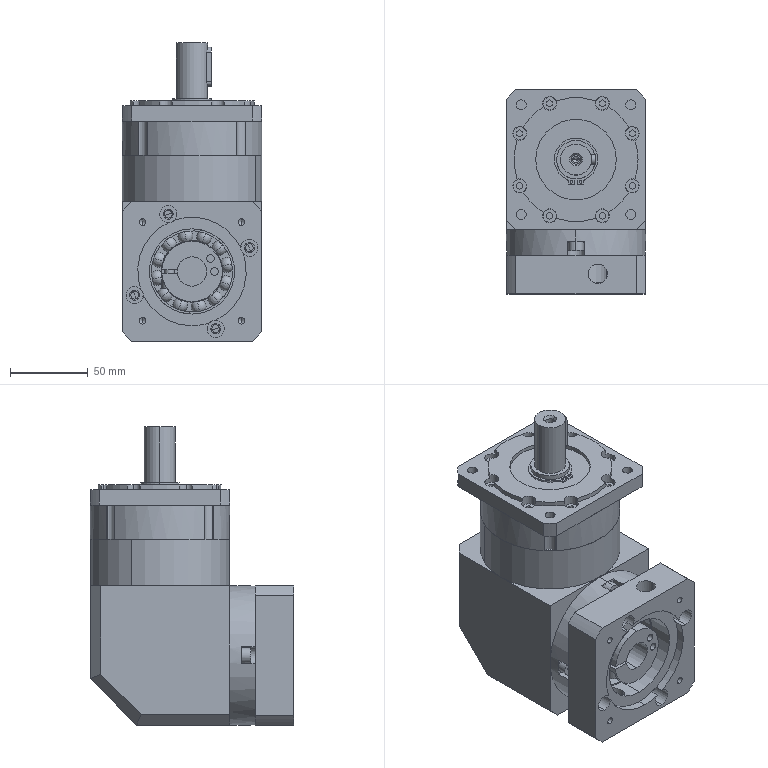Part | SolidWorks | features BaseBody 8 | 8 solids | 664 faces | box 90 x 131.5 x 192.5 mm | volume 1289252 mm3 | plane 237 | cylinder 227 | sphere 96 | torus 90 | cone 14 | commonest cylinder face diameters 5 x16 6.5 x16 8.5 x16 9 x16 10 x16 11 x14